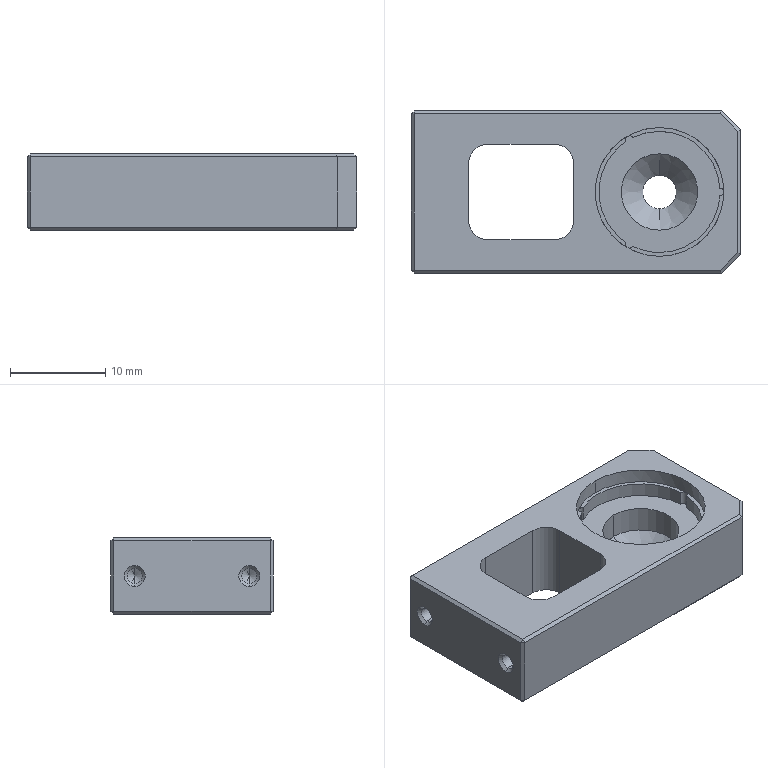NC program | NX | posted with a generic post | part box 34.5 x 17 x 8 mm
Lines 1 to 1240 of 4112:
N10 G17 G21 G94 G90
(FLOOR_WALL , TOOL : D10JING)
N12 T09 M6
N14 G54
N16 G17 G0 G90 X-27.25 Y10.497 S9500 M3
N18 G43 Z30. H9
N20 Z3.
N22 G94 G1 Z0. F1250.
N24 X-24.25
N26 X24.25
N28 Y6.248
N30 X-24.25
N32 Y1.999
N34 X24.25
N36 Y-2.251
N38 X-24.25
N40 Y-6.5
N42 X24.25
N44 X27.25
N46 Z3.
N48 G0 Z30.
N50 M5
(ZLEVEL_PROFILE , TOOL : D10)
N52 T10 M6
N54 G54
N56 G17 G0 G90 X-12.343 Y-13.6 S9500 M3
N58 G43 Z30. H10
N60 Z1.5
N62 G94 G1 X-17.504 Z1.23 F1000.
N64 X-18.913 Y-13.24 Z1.153
N66 X-20.165 Y-12.498 Z1.077
N68 X-21.248 Y-11.415 Z0.997
N70 X-21.99 Y-10.163 Z0.921
N72 X-22.35 Y-8.754 Z0.844
N74 Y8.754 Z-0.073
N76 X-21.99 Y10.163 Z-0.149
N78 X-21.248 Y11.415 Z-0.226
N80 X-20.165 Y12.498 Z-0.306
N82 X-18.913 Y13.24 Z-0.382
N84 X-17.504 Y13.6 Z-0.458
N86 X-16.95 Z-0.488
N88 X15.25 F2500.
N90 G2 X18.856 Y12.106 R5.1
N92 G1 X20.856 Y10.106
N94 G2 X22.35 Y6.5 R5.1
N96 G1 Y-6.5
N98 G2 X20.856 Y-10.106 R5.1
N100 G1 X18.856 Y-12.106
N102 G2 X15.25 Y-13.6 R5.1
N104 G1 X-16.95
N106 G2 X-20.556 Y-12.106 R5.1
N108 G1 X-20.856 Y-11.806
N110 G2 X-22.35 Y-8.2 R5.1
N112 G1 Y8.2
N114 G2 X-20.856 Y11.806 R5.1
N116 G1 X-20.556 Y12.106
N118 G2 X-16.95 Y13.6 R5.1
N120 G1 X10.979 Z-0.975
N122 X15.25
N124 G2 X18.856 Y12.106 R5.1
N126 G1 X20.856 Y10.106
N128 G2 X22.35 Y6.5 R5.1
N130 G1 Y-6.5
N132 G2 X20.856 Y-10.106 R5.1
N134 G1 X18.856 Y-12.106
N136 G2 X15.25 Y-13.6 R5.1
N138 G1 X-16.95
N140 G2 X-20.556 Y-12.106 R5.1
N142 G1 X-20.856 Y-11.806
N144 G2 X-22.35 Y-8.2 R5.1
N146 G1 Y8.2
N148 G2 X-20.856 Y11.806 R5.1
N150 G1 X-20.556 Y12.106
N152 G2 X-16.95 Y13.6 R5.1
N154 G1 X10.979 Z-1.463
N156 X15.25
N158 G2 X18.856 Y12.106 R5.1
N160 G1 X20.856 Y10.106
N162 G2 X22.35 Y6.5 R5.1
N164 G1 Y-6.5
N166 G2 X20.856 Y-10.106 R5.1
N168 G1 X18.856 Y-12.106
N170 G2 X15.25 Y-13.6 R5.1
N172 G1 X-16.95
N174 G2 X-20.556 Y-12.106 R5.1
N176 G1 X-20.856 Y-11.806
N178 G2 X-22.35 Y-8.2 R5.1
N180 G1 Y8.2
N182 G2 X-20.856 Y11.806 R5.1
N184 G1 X-20.556 Y12.106
N186 G2 X-16.95 Y13.6 R5.1
N188 G1 X10.979 Z-1.95
N190 X15.25
N192 G2 X18.856 Y12.106 R5.1
N194 G1 X20.856 Y10.106
N196 G2 X22.35 Y6.5 R5.1
N198 G1 Y-6.5
N200 G2 X20.856 Y-10.106 R5.1
N202 G1 X18.856 Y-12.106
N204 G2 X15.25 Y-13.6 R5.1
N206 G1 X-16.95
N208 G2 X-20.556 Y-12.106 R5.1
N210 G1 X-20.856 Y-11.806
N212 G2 X-22.35 Y-8.2 R5.1
N214 G1 Y8.2
N216 G2 X-20.856 Y11.806 R5.1
N218 G1 X-20.556 Y12.106
N220 G2 X-16.95 Y13.6 R5.1
N222 G1 X10.979 Z-2.438
N224 X15.25
N226 G2 X18.856 Y12.106 R5.1
N228 G1 X20.856 Y10.106
N230 G2 X22.35 Y6.5 R5.1
N232 G1 Y-6.5
N234 G2 X20.856 Y-10.106 R5.1
N236 G1 X18.856 Y-12.106
N238 G2 X15.25 Y-13.6 R5.1
N240 G1 X-16.95
N242 G2 X-20.556 Y-12.106 R5.1
N244 G1 X-20.856 Y-11.806
N246 G2 X-22.35 Y-8.2 R5.1
N248 G1 Y8.2
N250 G2 X-20.856 Y11.806 R5.1
N252 G1 X-20.556 Y12.106
N254 G2 X-16.95 Y13.6 R5.1
N256 G1 X10.979 Z-2.925
N258 X15.25
N260 G2 X18.856 Y12.106 R5.1
N262 G1 X20.856 Y10.106
N264 G2 X22.35 Y6.5 R5.1
N266 G1 Y-6.5
N268 G2 X20.856 Y-10.106 R5.1
N270 G1 X18.856 Y-12.106
N272 G2 X15.25 Y-13.6 R5.1
N274 G1 X-16.95
N276 G2 X-20.556 Y-12.106 R5.1
N278 G1 X-20.856 Y-11.806
N280 G2 X-22.35 Y-8.2 R5.1
N282 G1 Y8.2
N284 G2 X-20.856 Y11.806 R5.1
N286 G1 X-20.556 Y12.106
N288 G2 X-16.95 Y13.6 R5.1
N290 G1 X10.979 Z-3.413
N292 X15.25
N294 G2 X18.856 Y12.106 R5.1
N296 G1 X20.856 Y10.106
N298 G2 X22.35 Y6.5 R5.1
N300 G1 Y-6.5
N302 G2 X20.856 Y-10.106 R5.1
N304 G1 X18.856 Y-12.106
N306 G2 X15.25 Y-13.6 R5.1
N308 G1 X-16.95
N310 G2 X-20.556 Y-12.106 R5.1
N312 G1 X-20.856 Y-11.806
N314 G2 X-22.35 Y-8.2 R5.1
N316 G1 Y8.2
N318 G2 X-20.856 Y11.806 R5.1
N320 G1 X-20.556 Y12.106
N322 G2 X-16.95 Y13.6 R5.1
N324 G1 X10.979 Z-3.9
N326 X15.25
N328 G2 X18.856 Y12.106 R5.1
N330 G1 X20.856 Y10.106
N332 G2 X22.35 Y6.5 R5.1
N334 G1 Y-6.5
N336 G2 X20.856 Y-10.106 R5.1
N338 G1 X18.856 Y-12.106
N340 G2 X15.25 Y-13.6 R5.1
N342 G1 X-16.95
N344 G2 X-20.556 Y-12.106 R5.1
N346 G1 X-20.856 Y-11.806
N348 G2 X-22.35 Y-8.2 R5.1
N350 G1 Y8.2
N352 G2 X-20.856 Y11.806 R5.1
N354 G1 X-20.556 Y12.106
N356 G2 X-16.95 Y13.6 R5.1
N358 G1 X10.979 Z-4.388
N360 X15.25
N362 G2 X18.856 Y12.106 R5.1
N364 G1 X20.856 Y10.106
N366 G2 X22.35 Y6.5 R5.1
N368 G1 Y-6.5
N370 G2 X20.856 Y-10.106 R5.1
N372 G1 X18.856 Y-12.106
N374 G2 X15.25 Y-13.6 R5.1
N376 G1 X-16.95
N378 G2 X-20.556 Y-12.106 R5.1
N380 G1 X-20.856 Y-11.806
N382 G2 X-22.35 Y-8.2 R5.1
N384 G1 Y8.2
N386 G2 X-20.856 Y11.806 R5.1
N388 G1 X-20.556 Y12.106
N390 G2 X-16.95 Y13.6 R5.1
N392 G1 X10.979 Z-4.875
N394 X15.25
N396 G2 X18.856 Y12.106 R5.1
N398 G1 X20.856 Y10.106
N400 G2 X22.35 Y6.5 R5.1
N402 G1 Y-6.5
N404 G2 X20.856 Y-10.106 R5.1
N406 G1 X18.856 Y-12.106
N408 G2 X15.25 Y-13.6 R5.1
N410 G1 X-16.95
N412 G2 X-20.556 Y-12.106 R5.1
N414 G1 X-20.856 Y-11.806
N416 G2 X-22.35 Y-8.2 R5.1
N418 G1 Y8.2
N420 G2 X-20.856 Y11.806 R5.1
N422 G1 X-20.556 Y12.106
N424 G2 X-16.95 Y13.6 R5.1
N426 G1 X10.979 Z-5.363
N428 X15.25
N430 G2 X18.856 Y12.106 R5.1
N432 G1 X20.856 Y10.106
N434 G2 X22.35 Y6.5 R5.1
N436 G1 Y-6.5
N438 G2 X20.856 Y-10.106 R5.1
N440 G1 X18.856 Y-12.106
N442 G2 X15.25 Y-13.6 R5.1
N444 G1 X-16.95
N446 G2 X-20.556 Y-12.106 R5.1
N448 G1 X-20.856 Y-11.806
N450 G2 X-22.35 Y-8.2 R5.1
N452 G1 Y8.2
N454 G2 X-20.856 Y11.806 R5.1
N456 G1 X-20.556 Y12.106
N458 G2 X-16.95 Y13.6 R5.1
N460 G1 X10.979 Z-5.85
N462 X15.25
N464 G2 X18.856 Y12.106 R5.1
N466 G1 X20.856 Y10.106
N468 G2 X22.35 Y6.5 R5.1
N470 G1 Y-6.5
N472 G2 X20.856 Y-10.106 R5.1
N474 G1 X18.856 Y-12.106
N476 G2 X15.25 Y-13.6 R5.1
N478 G1 X-16.95
N480 G2 X-20.556 Y-12.106 R5.1
N482 G1 X-20.856 Y-11.806
N484 G2 X-22.35 Y-8.2 R5.1
N486 G1 Y8.2
N488 G2 X-20.856 Y11.806 R5.1
N490 G1 X-20.556 Y12.106
N492 G2 X-16.95 Y13.6 R5.1
N494 G1 X10.979 Z-6.338
N496 X15.25
N498 G2 X18.856 Y12.106 R5.1
N500 G1 X20.856 Y10.106
N502 G2 X22.35 Y6.5 R5.1
N504 G1 Y-6.5
N506 G2 X20.856 Y-10.106 R5.1
N508 G1 X18.856 Y-12.106
N510 G2 X15.25 Y-13.6 R5.1
N512 G1 X-16.95
N514 G2 X-20.556 Y-12.106 R5.1
N516 G1 X-20.856 Y-11.806
N518 G2 X-22.35 Y-8.2 R5.1
N520 G1 Y8.2
N522 G2 X-20.856 Y11.806 R5.1
N524 G1 X-20.556 Y12.106
N526 G2 X-16.95 Y13.6 R5.1
N528 G1 X10.979 Z-6.825
N530 X15.25
N532 G2 X18.856 Y12.106 R5.1
N534 G1 X20.856 Y10.106
N536 G2 X22.35 Y6.5 R5.1
N538 G1 Y-6.5
N540 G2 X20.856 Y-10.106 R5.1
N542 G1 X18.856 Y-12.106
N544 G2 X15.25 Y-13.6 R5.1
N546 G1 X-16.95
N548 G2 X-20.556 Y-12.106 R5.1
N550 G1 X-20.856 Y-11.806
N552 G2 X-22.35 Y-8.2 R5.1
N554 G1 Y8.2
N556 G2 X-20.856 Y11.806 R5.1
N558 G1 X-20.556 Y12.106
N560 G2 X-16.95 Y13.6 R5.1
N562 G1 X10.979 Z-7.313
N564 X15.25
N566 G2 X18.856 Y12.106 R5.1
N568 G1 X20.856 Y10.106
N570 G2 X22.35 Y6.5 R5.1
N572 G1 Y-6.5
N574 G2 X20.856 Y-10.106 R5.1
N576 G1 X18.856 Y-12.106
N578 G2 X15.25 Y-13.6 R5.1
N580 G1 X-16.95
N582 G2 X-20.556 Y-12.106 R5.1
N584 G1 X-20.856 Y-11.806
N586 G2 X-22.35 Y-8.2 R5.1
N588 G1 Y8.2
N590 G2 X-20.856 Y11.806 R5.1
N592 G1 X-20.556 Y12.106
N594 G2 X-16.95 Y13.6 R5.1
N596 G1 X10.979 Z-7.8
N598 X15.25
N600 G2 X18.856 Y12.106 R5.1
N602 G1 X20.856 Y10.106
N604 G2 X22.35 Y6.5 R5.1
N606 G1 Y-6.5
N608 G2 X20.856 Y-10.106 R5.1
N610 G1 X18.856 Y-12.106
N612 G2 X15.25 Y-13.6 R5.1
N614 G1 X-16.95
N616 G2 X-20.556 Y-12.106 R5.1
N618 G1 X-20.856 Y-11.806
N620 G2 X-22.35 Y-8.2 R5.1
N622 G1 Y8.2
N624 G2 X-20.856 Y11.806 R5.1
N626 G1 X-20.556 Y12.106
N628 G2 X-16.95 Y13.6 R5.1
N630 G1 X10.979
N632 Z-6.3
N634 G0 Z30.
(HOLE_MILLING , TOOL : D10)
N636 X8.75 Y0.
N638 Z0.5
N640 G3 X9.575 Y-0.825 R0.825 F2000.
N642 X10.4 Y0. R0.825
N644 X10.4 Y0. Z0. I-1.65 J0.
N646 X10.4 Y0. Z-0.5 I-1.65 J0.
N648 X10.4 Y0. Z-1. I-1.65 J0.
N650 X10.4 Y0. Z-1.5 I-1.65 J0.
N652 X8.75 Y1.65 R1.65
N654 X10.4 Y0. R-1.65
N656 X9.575 Y0.825 R0.825
N658 X8.75 Y0. R0.825
N660 G0 Z30.
(HOLE_MILLING_COPY , TOOL : D10)
N662 Z-1.
N664 G3 X9.375 Y-0.625 R0.625
N666 X10. Y0. R0.625
N668 X10. Y0. Z-1.5 I-1.25 J0.
N670 X10. Y0. Z-2. I-1.25 J0.
N672 X10. Y0. Z-2.5 I-1.25 J0.
N674 X10. Y0. Z-3. I-1.25 J0.
N676 X8.75 Y1.25 R1.25
N678 X10. Y0. R-1.25
N680 X9.375 Y0.625 R0.625
N682 X8.75 Y0. R0.625
N684 G0 Z30.
N686 M5
(ZLEVEL_PROFILE_COPY_COPY , TOOL : D4)
N688 T04 M6
N690 G54
N692 G17 G0 G90 X-3.25 Y1.754 S9500 M3
N694 G43 Z30. H4
N696 Z1.5
N698 G94 G1 Y2.002 Z1.487 F1000.
N700 X-3.298 Y2. Z1.485
N702 X-8.202 Z1.227
N704 X-8.25 Y2.002 Z1.225
N706 Y-2. Z1.015
N708 X-3.25 Z0.753
N710 Y2.002 Z0.544
N712 X-3.298 Y2. Z0.541
N714 X-8.202 Z0.284
N716 X-8.25 Y2.002 Z0.281
N718 Y-2. Z0.072
N720 X-3.25 Z-0.19
N722 Y2.002 Z-0.4
N724 X-3.298 Y2. F2000.
N726 X-8.202
N728 X-8.25 Y2.002
N730 Y-2.
N732 X-3.25
N734 Y2.002
N736 X-3.423 Y2. Z-0.405
N738 X-8.097 Z-0.544
N740 X-8.25 Y1.982 Z-0.549
N742 Y-2. Z-0.667
N744 X-8.077 Z-0.672
N746 X-3.749 Z-0.8
N748 X-3.25
N750 Y2.002
N752 X-3.423 Y2. Z-0.805
N754 X-8.097 Z-0.944
N756 X-8.25 Y1.982 Z-0.949
N758 Y-2. Z-1.067
N760 X-8.077 Z-1.072
N762 X-3.749 Z-1.2
N764 X-3.25
N766 Y2.002
N768 X-3.423 Y2. Z-1.205
N770 X-8.097 Z-1.344
N772 X-8.25 Y1.982 Z-1.349
N774 Y-2. Z-1.467
N776 X-8.077 Z-1.472
N778 X-3.749 Z-1.6
N780 X-3.25
N782 Y2.002
N784 X-3.423 Y2. Z-1.605
N786 X-8.097 Z-1.744
N788 X-8.25 Y1.982 Z-1.749
N790 Y-2. Z-1.867
N792 X-8.077 Z-1.872
N794 X-3.749 Z-2.
N796 X-3.25
N798 Y2.002
N800 X-3.423 Y2. Z-2.005
N802 X-8.097 Z-2.144
N804 X-8.25 Y1.982 Z-2.149
N806 Y-2. Z-2.267
N808 X-8.077 Z-2.272
N810 X-3.749 Z-2.4
N812 X-3.25
N814 Y2.002
N816 X-3.423 Y2. Z-2.405
N818 X-8.097 Z-2.544
N820 X-8.25 Y1.982 Z-2.549
N822 Y-2. Z-2.667
N824 X-8.077 Z-2.672
N826 X-3.749 Z-2.8
N828 X-3.25
N830 Y2.002
N832 X-3.423 Y2. Z-2.805
N834 X-8.097 Z-2.944
N836 X-8.25 Y1.982 Z-2.949
N838 Y-2. Z-3.067
N840 X-8.077 Z-3.072
N842 X-3.749 Z-3.2
N844 X-3.25
N846 Y2.002
N848 X-3.423 Y2. Z-3.205
N850 X-8.097 Z-3.344
N852 X-8.25 Y1.982 Z-3.349
N854 Y-2. Z-3.467
N856 X-8.077 Z-3.472
N858 X-3.749 Z-3.6
N860 X-3.25
N862 Y2.002
N864 X-3.423 Y2. Z-3.605
N866 X-8.097 Z-3.744
N868 X-8.25 Y1.982 Z-3.749
N870 Y-2. Z-3.867
N872 X-8.077 Z-3.872
N874 X-3.749 Z-4.
N876 X-3.25
N878 Y2.002
N880 X-3.423 Y2. Z-4.005
N882 X-8.097 Z-4.144
N884 X-8.25 Y1.982 Z-4.149
N886 Y-2. Z-4.267
N888 X-8.077 Z-4.272
N890 X-3.749 Z-4.4
N892 X-3.25
N894 Y2.002
N896 X-3.423 Y2. Z-4.405
N898 X-8.097 Z-4.544
N900 X-8.25 Y1.982 Z-4.549
N902 Y-2. Z-4.667
N904 X-8.077 Z-4.672
N906 X-3.749 Z-4.8
N908 X-3.25
N910 Y2.002
N912 X-3.423 Y2. Z-4.805
N914 X-8.097 Z-4.944
N916 X-8.25 Y1.982 Z-4.949
N918 Y-2. Z-5.067
N920 X-8.077 Z-5.072
N922 X-3.749 Z-5.2
N924 X-3.25
N926 Y2.002
N928 X-3.423 Y2. Z-5.205
N930 X-8.097 Z-5.344
N932 X-8.25 Y1.982 Z-5.349
N934 Y-2. Z-5.467
N936 X-8.077 Z-5.472
N938 X-3.749 Z-5.6
N940 X-3.25
N942 Y2.002
N944 X-3.423 Y2. Z-5.605
N946 X-8.097 Z-5.744
N948 X-8.25 Y1.982 Z-5.749
N950 Y-2. Z-5.867
N952 X-8.077 Z-5.872
N954 X-3.749 Z-6.
N956 X-3.25
N958 Y2.002
N960 X-3.423 Y2. Z-6.005
N962 X-8.097 Z-6.144
N964 X-8.25 Y1.982 Z-6.149
N966 Y-2. Z-6.267
N968 X-8.077 Z-6.272
N970 X-3.749 Z-6.4
N972 X-3.25
N974 Y2.002
N976 X-3.423 Y2. Z-6.405
N978 X-8.097 Z-6.544
N980 X-8.25 Y1.982 Z-6.549
N982 Y-2. Z-6.667
N984 X-8.077 Z-6.672
N986 X-3.749 Z-6.8
N988 X-3.25
N990 Y2.002
N992 X-3.423 Y2. Z-6.805
N994 X-8.097 Z-6.944
N996 X-8.25 Y1.981 Z-6.949
N998 Y-2. Z-7.067
N1000 X-8.077 Z-7.072
N1002 X-3.749 Z-7.2
N1004 X-3.25
N1006 Y2.002
N1008 X-3.423 Y2. Z-7.205
N1010 X-8.097 Z-7.344
N1012 X-8.25 Y1.981 Z-7.349
N1014 Y-2. Z-7.467
N1016 X-8.077 Z-7.472
N1018 X-3.749 Z-7.6
N1020 X-3.25
N1022 Y2.002
N1024 X-3.423 Y2. Z-7.605
N1026 X-8.097 Z-7.744
N1028 X-8.25 Y1.981 Z-7.749
N1030 Y-2. Z-7.867
N1032 X-8.077 Z-7.872
N1034 X-3.749 Z-8.
N1036 X-3.25
N1038 Y2.002
N1040 X-3.298 Y2.
N1042 X-8.202
N1044 X-8.25 Y2.002
N1046 Y-2.
N1048 X-3.749
N1050 Z-6.5
N1052 G0 Z30.
(ZLEVEL_PROFILE_COPY_COPY_COPY , TOOL : D4)
N1054 X-7.596 Y-2.9
N1056 Z1.5
N1058 G1 X-2.35 Z1.225 F1000.
N1060 Y2.903 Z0.921
N1062 X-2.39 Y2.9 Z0.919
N1064 X-9.11 Z0.567
N1066 X-9.15 Y2.903 Z0.565
N1068 Y-2.9 Z0.26
N1070 X-2.35 Z-0.096
N1072 Y2.903 Z-0.4
N1074 X-2.39 Y2.9 F2000.
N1076 X-9.11
N1078 X-9.15 Y2.903
N1080 Y-2.9
N1082 X-2.35
N1084 Y2.903
N1086 X-2.494 Y2.9 Z-0.403
N1088 X-8.988 Z-0.54
N1090 X-9.132 Y2.901 Z-0.544
N1092 X-9.15 Y2.776 Z-0.547
N1094 Y-2.852 Z-0.666
N1096 X-9.054 Y-2.9 Z-0.669
N1098 X-2.849 Z-0.8
N1100 X-2.35
N1102 Y2.903
N1104 X-2.494 Y2.9 Z-0.803
N1106 X-8.988 Z-0.94
N1108 X-9.132 Y2.901 Z-0.944
N1110 X-9.15 Y2.776 Z-0.947
N1112 Y-2.852 Z-1.066
N1114 X-9.054 Y-2.9 Z-1.069
N1116 X-2.849 Z-1.2
N1118 X-2.35
N1120 Y2.903
N1122 X-2.494 Y2.9 Z-1.203
N1124 X-8.988 Z-1.34
N1126 X-9.132 Y2.901 Z-1.344
N1128 X-9.15 Y2.776 Z-1.347
N1130 Y-2.852 Z-1.466
N1132 X-9.054 Y-2.9 Z-1.469
N1134 X-2.849 Z-1.6
N1136 X-2.35
N1138 Y2.902
N1140 X-2.494 Y2.9 Z-1.603
N1142 X-8.988 Z-1.74
N1144 X-9.132 Y2.901 Z-1.744
N1146 X-9.15 Y2.776 Z-1.747
N1148 Y-2.852 Z-1.866
N1150 X-9.054 Y-2.9 Z-1.869
N1152 X-2.849 Z-2.
N1154 X-2.35
N1156 Y2.902
N1158 X-2.494 Y2.9 Z-2.003
N1160 X-8.988 Z-2.14
N1162 X-9.132 Y2.901 Z-2.144
N1164 X-9.15 Y2.776 Z-2.147
N1166 Y-2.852 Z-2.266
N1168 X-9.054 Y-2.9 Z-2.269
N1170 X-2.849 Z-2.4
N1172 X-2.35
N1174 Y2.902
N1176 X-2.494 Y2.9 Z-2.403
N1178 X-8.988 Z-2.54
N1180 X-9.132 Y2.901 Z-2.544
N1182 X-9.15 Y2.776 Z-2.547
N1184 Y-2.852 Z-2.666
N1186 X-9.054 Y-2.9 Z-2.669
N1188 X-2.849 Z-2.8
N1190 X-2.35
N1192 Y2.902
N1194 X-2.494 Y2.9 Z-2.803
N1196 X-8.988 Z-2.94
N1198 X-9.132 Y2.901 Z-2.944
N1200 X-9.15 Y2.776 Z-2.947
N1202 Y-2.852 Z-3.066
N1204 X-9.054 Y-2.9 Z-3.069
N1206 X-2.849 Z-3.2
N1208 X-2.35
N1210 Y2.902
N1212 X-2.494 Y2.9 Z-3.203
N1214 X-8.988 Z-3.34
N1216 X-9.132 Y2.901 Z-3.344
N1218 X-9.15 Y2.776 Z-3.347
N1220 Y-2.852 Z-3.466
N1222 X-9.054 Y-2.9 Z-3.469
N1224 X-2.849 Z-3.6
N1226 X-2.35
N1228 Y2.902
N1230 X-2.494 Y2.9 Z-3.603
N1232 X-8.988 Z-3.74
N1234 X-9.132 Y2.901 Z-3.744
N1236 X-9.15 Y2.776 Z-3.747
N1238 Y-2.852 Z-3.866
N1240 X-9.054 Y-2.9 Z-3.869
N1242 X-2.849 Z-4.
N1244 X-2.35
N1246 Y2.902
N1248 X-2.494 Y2.9 Z-4.003
N1250 X-8.988 Z-4.14
N1252 X-9.132 Y2.901 Z-4.144
N1254 X-9.15 Y2.776 Z-4.147
N1256 Y-2.852 Z-4.266
N1258 X-9.054 Y-2.9 Z-4.269
N1260 X-2.849 Z-4.4
N1262 X-2.35
N1264 Y2.902
N1266 X-2.494 Y2.9 Z-4.403
N1268 X-8.988 Z-4.54
N1270 X-9.132 Y2.901 Z-4.544
N1272 X-9.15 Y2.776 Z-4.547
N1274 Y-2.852 Z-4.666
N1276 X-9.054 Y-2.9 Z-4.669
N1278 X-2.849 Z-4.8
N1280 X-2.35
N1282 Y2.902
N1284 X-2.494 Y2.9 Z-4.803
N1286 X-8.988 Z-4.94
N1288 X-9.132 Y2.901 Z-4.944
N1290 X-9.15 Y2.776 Z-4.947
N1292 Y-2.852 Z-5.066
N1294 X-9.054 Y-2.9 Z-5.069
N1296 X-2.849 Z-5.2
N1298 X-2.35
N1300 Y2.902
N1302 X-2.494 Y2.9 Z-5.203
N1304 X-8.988 Z-5.34
N1306 X-9.132 Y2.901 Z-5.344
N1308 X-9.15 Y2.776 Z-5.347
N1310 Y-2.852 Z-5.466
N1312 X-9.054 Y-2.9 Z-5.469
N1314 X-2.849 Z-5.6
N1316 X-2.35
N1318 Y2.902
N1320 X-2.494 Y2.9 Z-5.603
N1322 X-8.988 Z-5.74
N1324 X-9.132 Y2.901 Z-5.744
N1326 X-9.15 Y2.776 Z-5.747
N1328 Y-2.852 Z-5.866
N1330 X-9.054 Y-2.9 Z-5.869
N1332 X-2.849 Z-6.
N1334 X-2.35
N1336 Y2.902
N1338 X-2.494 Y2.9 Z-6.003
N1340 X-8.988 Z-6.14
N1342 X-9.132 Y2.901 Z-6.144
N1344 X-9.15 Y2.776 Z-6.147
N1346 Y-2.852 Z-6.266
N1348 X-9.054 Y-2.9 Z-6.269
N1350 X-2.849 Z-6.4
N1352 X-2.35
N1354 Y2.902
N1356 X-2.494 Y2.9 Z-6.403
N1358 X-8.988 Z-6.54
N1360 X-9.132 Y2.901 Z-6.544
N1362 X-9.15 Y2.776 Z-6.547
N1364 Y-2.852 Z-6.666
N1366 X-9.054 Y-2.9 Z-6.669
N1368 X-2.849 Z-6.8
N1370 X-2.35
N1372 Y2.902
N1374 X-2.494 Y2.9 Z-6.803
N1376 X-8.988 Z-6.94
N1378 X-9.132 Y2.901 Z-6.944
N1380 X-9.15 Y2.776 Z-6.947
N1382 Y-2.852 Z-7.066
N1384 X-9.054 Y-2.9 Z-7.069
N1386 X-2.849 Z-7.2
N1388 X-2.35
N1390 Y2.902
N1392 X-2.494 Y2.9 Z-7.203
N1394 X-8.988 Z-7.34
N1396 X-9.132 Y2.901 Z-7.344
N1398 X-9.15 Y2.776 Z-7.347
N1400 Y-2.852 Z-7.466
N1402 X-9.054 Y-2.9 Z-7.469
N1404 X-2.849 Z-7.6
N1406 X-2.35
N1408 Y2.902
N1410 X-2.494 Y2.9 Z-7.603
N1412 X-8.988 Z-7.74
N1414 X-9.132 Y2.901 Z-7.744
N1416 X-9.15 Y2.776 Z-7.747
N1418 Y-2.852 Z-7.866
N1420 X-9.054 Y-2.9 Z-7.869
N1422 X-2.849 Z-8.
N1424 X-2.35
N1426 Y2.902
N1428 X-2.39 Y2.9
N1430 X-9.11
N1432 X-9.15 Y2.902
N1434 Y-2.9
N1436 X-2.849
N1438 Z-6.5
N1440 G0 Z30.
(ZLEVEL_PROFILE_COPY_COPY_COPY_COPY_1 , TOOL : D4)
N1442 X9.088 Y1.869
N1444 Z-1.5
N1446 G1 X8.949 Y1.9 Z-1.507 F1000.
N1448 X8.75 Z-1.518
N1450 X8.555 Z-1.528
N1452 X8.12 Y1.803 Z-1.551
N1454 X7.719 Y1.608 Z-1.575
N1456 X7.375 Y1.326 Z-1.598
N1458 X7.105 Y0.971 Z-1.622
N1460 X6.942 Y0.616 Z-1.642
N1462 X6.845 Y0.136 Z-1.668
N1464 X6.873 Y-0.352 Z-1.693
N1466 X7.024 Y-0.818 Z-1.719
N1468 X7.289 Y-1.23 Z-1.745
N1470 X7.649 Y-1.561 Z-1.77
N1472 X8.082 Y-1.789 Z-1.796
N1474 X8.559 Y-1.9 Z-1.822
N1476 X8.949 Z-1.842
N1478 X9.434 Y-1.783 Z-1.868
N1480 X9.873 Y-1.545 Z-1.894
N1482 X10.235 Y-1.201 Z-1.92
N1484 X10.495 Y-0.776 Z-1.947
N1486 X10.637 Y-0.297 Z-1.973
N1488 X10.649 Y0.202 Z-1.999
N1490 X10.532 Y0.687 Z-2.025
N1492 X10.355 Y1.035 Z-2.046
N1494 X10.086 Y1.365 Z-2.068
N1496 X9.75 Y1.627 Z-2.09
N1498 X9.365 Y1.808 Z-2.112
N1500 X8.949 Y1.9 Z-2.135
N1502 X8.75 Z-2.145
N1504 X8.555 Z-2.155
N1506 X8.12 Y1.803 Z-2.179
N1508 X7.719 Y1.608 Z-2.202
N1510 X7.375 Y1.326 Z-2.226
N1512 X7.105 Y0.971 Z-2.249
N1514 X6.942 Y0.616 Z-2.269
N1516 X6.845 Y0.136 Z-2.295
N1518 X6.873 Y-0.352 Z-2.321
N1520 X7.024 Y-0.818 Z-2.346
N1522 X7.289 Y-1.23 Z-2.372
N1524 X7.649 Y-1.561 Z-2.398
N1526 X8.082 Y-1.789 Z-2.423
N1528 X8.559 Y-1.9 Z-2.449
N1530 X8.949 Z-2.469
N1532 X9.434 Y-1.783 Z-2.496
N1534 X9.873 Y-1.545 Z-2.522
N1536 X10.235 Y-1.201 Z-2.548
N1538 X10.495 Y-0.776 Z-2.574
N1540 X10.637 Y-0.297 Z-2.6
N1542 X10.649 Y0.202 Z-2.626
N1544 X10.532 Y0.687 Z-2.652
N1546 X10.355 Y1.035 Z-2.673
N1548 X10.086 Y1.365 Z-2.695
N1550 X9.75 Y1.627 Z-2.718
N1552 X9.365 Y1.808 Z-2.74
N1554 X8.949 Y1.9 Z-2.762
N1556 X8.75 Z-2.773
N1558 X8.555 Z-2.783
N1560 X8.12 Y1.803 Z-2.806
N1562 X7.719 Y1.608 Z-2.83
N1564 X7.375 Y1.326 Z-2.853
N1566 X7.105 Y0.971 Z-2.876
N1568 X6.942 Y0.616 Z-2.897
N1570 X6.845 Y0.136 Z-2.922
N1572 X6.873 Y-0.352 Z-2.948
N1574 X7.024 Y-0.818 Z-2.974
N1576 X7.289 Y-1.23 Z-2.999
N1578 X7.649 Y-1.561 Z-3.025
N1580 X8.082 Y-1.789 Z-3.051
N1582 X8.559 Y-1.9 Z-3.076
N1584 X8.949 Z-3.097
N1586 X9.434 Y-1.783 Z-3.123
N1588 X9.873 Y-1.545 Z-3.149
N1590 X10.235 Y-1.201 Z-3.175
N1592 X10.495 Y-0.776 Z-3.201
N1594 X10.637 Y-0.297 Z-3.228
N1596 X10.649 Y0.202 Z-3.254
N1598 X10.532 Y0.687 Z-3.28
N1600 X10.355 Y1.035 Z-3.3
N1602 X10.086 Y1.365 Z-3.323
N1604 X9.75 Y1.627 Z-3.345
N1606 X9.365 Y1.808 Z-3.367
N1608 X8.949 Y1.9 Z-3.39
N1610 X8.75 Z-3.4
N1612 G3 X6.85 Y0. R1.9 F2000.
N1614 X8.75 Y1.9 R-1.9
N1616 G1 X8.607 Y1.885 Z-3.406
N1618 X8.463 Y1.872 Z-3.413
N1620 X8.322 Y1.843 Z-3.419
N1622 X8.184 Y1.805 Z-3.426
N1624 X8.048 Y1.757 Z-3.432
N1626 X7.917 Y1.698 Z-3.439
N1628 X7.789 Y1.632 Z-3.445
N1630 X7.67 Y1.552 Z-3.452
N1632 X7.552 Y1.469 Z-3.458
N1634 X7.447 Y1.37 Z-3.465
N1636 X7.345 Y1.269 Z-3.471
N1638 X7.254 Y1.158 Z-3.477
N1640 X7.17 Y1.041 Z-3.484
N1642 X7.095 Y0.918 Z-3.49
N1644 X7.032 Y0.79 Z-3.497
N1646 X6.974 Y0.658 Z-3.503
N1648 X6.932 Y0.52 Z-3.51
N1650 X6.894 Y0.381 Z-3.516
N1652 X6.874 Y0.239 Z-3.523
N1654 X6.859 Y0.096 Z-3.529
N1656 Y-0.048 Z-3.535
N1658 X6.868 Y-0.191 Z-3.542
N1660 X6.887 Y-0.334 Z-3.548
N1662 X6.919 Y-0.474 Z-3.555
N1664 X6.958 Y-0.612 Z-3.561
N1666 X7.012 Y-0.746 Z-3.568
N1668 X7.07 Y-0.877 Z-3.574
N1670 X7.145 Y-1. Z-3.581
N1672 X7.224 Y-1.12 Z-3.587
N1674 X7.315 Y-1.232 Z-3.594
N1676 X7.412 Y-1.338 Z-3.6
N1678 X7.517 Y-1.436 Z-3.606
N1680 X7.631 Y-1.525 Z-3.613
N1682 X7.748 Y-1.608 Z-3.619
N1684 X7.875 Y-1.676 Z-3.626
N1686 X8.003 Y-1.741 Z-3.632
N1688 X8.138 Y-1.789 Z-3.639
N1690 X8.275 Y-1.833 Z-3.645
N1692 X8.416 Y-1.862 Z-3.652
N1694 X8.559 Y-1.882 Z-3.658
N1696 X8.702 Y-1.892 Z-3.665
N1698 X8.846 Y-1.889 Z-3.671
N1700 X8.989 Y-1.879 Z-3.677
N1702 X9.131 Y-1.852 Z-3.684
N1704 X9.271 Y-1.821 Z-3.69
N1706 X9.407 Y-1.773 Z-3.697
N1708 X9.54 Y-1.72 Z-3.703
N1710 X9.668 Y-1.654 Z-3.71
N1712 X9.791 Y-1.58 Z-3.716
N1714 X9.908 Y-1.497 Z-3.723
N1716 X10.018 Y-1.403 Z-3.729
N1718 X10.123 Y-1.305 Z-3.735
N1720 X10.216 Y-1.195 Z-3.742
N1722 X10.305 Y-1.082 Z-3.748
N1724 X10.38 Y-0.959 Z-3.755
N1726 X10.45 Y-0.834 Z-3.761
N1728 X10.507 Y-0.702 Z-3.768
N1730 X10.555 Y-0.566 Z-3.774
N1732 X10.593 Y-0.428 Z-3.781
N1734 X10.619 Y-0.286 Z-3.787
N1736 X10.639 Y-0.143 Z-3.794
N1738 X10.65 Y0. Z-3.8
N1740 G3 X8.75 Y1.9 R1.9
N1742 G1 X8.607 Y1.886 Z-3.806
N1744 X8.463 Y1.872 Z-3.813
N1746 X8.323 Y1.842 Z-3.819
N1748 X8.184 Y1.805 Z-3.826
N1750 X8.048 Y1.757 Z-3.832
N1752 X7.917 Y1.698 Z-3.839
N1754 X7.79 Y1.632 Z-3.845
N1756 X7.67 Y1.552 Z-3.852
N1758 X7.552 Y1.469 Z-3.858
N1760 X7.447 Y1.37 Z-3.865
N1762 X7.345 Y1.269 Z-3.871
N1764 X7.254 Y1.158 Z-3.877
N1766 X7.17 Y1.041 Z-3.884
N1768 X7.095 Y0.918 Z-3.89
N1770 X7.032 Y0.789 Z-3.897
N1772 X6.974 Y0.658 Z-3.903
N1774 X6.932 Y0.52 Z-3.91
N1776 X6.894 Y0.381 Z-3.916
N1778 X6.875 Y0.239 Z-3.923
N1780 X6.859 Y0.096 Z-3.929
N1782 X6.86 Y-0.048 Z-3.935
N1784 X6.868 Y-0.191 Z-3.942
N1786 X6.888 Y-0.334 Z-3.948
N1788 X6.919 Y-0.474 Z-3.955
N1790 X6.958 Y-0.613 Z-3.961
N1792 X7.012 Y-0.746 Z-3.968
N1794 X7.07 Y-0.877 Z-3.974
N1796 X7.145 Y-1. Z-3.981
N1798 X7.224 Y-1.121 Z-3.987
N1800 X7.315 Y-1.232 Z-3.994
N1802 X7.412 Y-1.338 Z-4.
N1804 X7.517 Y-1.436 Z-4.006
N1806 X7.631 Y-1.524 Z-4.013
N1808 X7.748 Y-1.607 Z-4.019
N1810 X7.875 Y-1.676 Z-4.026
N1812 X8.003 Y-1.741 Z-4.032
N1814 X8.138 Y-1.789 Z-4.039
N1816 X8.276 Y-1.833 Z-4.045
N1818 X8.416 Y-1.862 Z-4.052
N1820 X8.559 Y-1.882 Z-4.058
N1822 X8.702 Y-1.892 Z-4.065
N1824 X8.846 Y-1.889 Z-4.071
N1826 X8.989 Y-1.879 Z-4.077
N1828 X9.131 Y-1.852 Z-4.084
N1830 X9.271 Y-1.821 Z-4.09
N1832 X9.407 Y-1.773 Z-4.097
N1834 X9.54 Y-1.72 Z-4.103
N1836 X9.668 Y-1.654 Z-4.11
N1838 X9.791 Y-1.579 Z-4.116
N1840 X9.908 Y-1.496 Z-4.123
N1842 X10.018 Y-1.403 Z-4.129
N1844 X10.123 Y-1.305 Z-4.135
N1846 X10.215 Y-1.195 Z-4.142
N1848 X10.305 Y-1.082 Z-4.148
N1850 X10.379 Y-0.959 Z-4.155
N1852 X10.45 Y-0.834 Z-4.161
N1854 X10.507 Y-0.702 Z-4.168
N1856 X10.555 Y-0.566 Z-4.174
N1858 X10.593 Y-0.428 Z-4.181
N1860 X10.619 Y-0.286 Z-4.187
N1862 X10.638 Y-0.143 Z-4.194
N1864 X10.65 Y0. Z-4.2
N1866 G3 X8.75 Y1.9 R1.9
N1868 G1 X8.607 Y1.886 Z-4.206
N1870 X8.463 Y1.872 Z-4.213
N1872 X8.323 Y1.842 Z-4.219
N1874 X8.184 Y1.805 Z-4.225
N1876 X8.048 Y1.757 Z-4.231
N1878 X7.917 Y1.698 Z-4.238
N1880 X7.79 Y1.632 Z-4.244
N1882 X7.67 Y1.552 Z-4.25
N1884 X7.553 Y1.469 Z-4.256
N1886 X7.447 Y1.37 Z-4.263
N1888 X7.345 Y1.269 Z-4.269
N1890 X7.254 Y1.158 Z-4.275
N1892 X7.171 Y1.041 Z-4.281
N1894 X7.095 Y0.918 Z-4.288
N1896 X7.032 Y0.789 Z-4.294
N1898 X6.974 Y0.658 Z-4.3
N1900 X6.932 Y0.52 Z-4.306
N1902 X6.894 Y0.381 Z-4.313
N1904 X6.875 Y0.239 Z-4.319
N1906 X6.859 Y0.096 Z-4.325
N1908 Y-0.048 Z-4.331
N1910 X6.868 Y-0.191 Z-4.338
N1912 X6.888 Y-0.334 Z-4.344
N1914 X6.919 Y-0.474 Z-4.35
N1916 X6.958 Y-0.613 Z-4.356
N1918 X7.013 Y-0.746 Z-4.363
N1920 X7.071 Y-0.877 Z-4.369
N1922 X7.146 Y-1. Z-4.375
N1924 X7.224 Y-1.121 Z-4.381
N1926 X7.315 Y-1.232 Z-4.388
N1928 X7.412 Y-1.338 Z-4.394
N1930 X7.517 Y-1.436 Z-4.4
N1932 X7.631 Y-1.524 Z-4.406
N1934 X7.748 Y-1.607 Z-4.413
N1936 X7.875 Y-1.676 Z-4.419
N1938 X8.003 Y-1.741 Z-4.425
N1940 X8.138 Y-1.789 Z-4.431
N1942 X8.276 Y-1.832 Z-4.438
N1944 X8.416 Y-1.862 Z-4.444
N1946 X8.559 Y-1.882 Z-4.45
N1948 X8.702 Y-1.892 Z-4.456
N1950 X8.846 Y-1.889 Z-4.463
N1952 X8.989 Y-1.879 Z-4.469
N1954 X9.131 Y-1.852 Z-4.475
N1956 X9.271 Y-1.821 Z-4.481
N1958 X9.407 Y-1.773 Z-4.488
N1960 X9.54 Y-1.72 Z-4.494
N1962 X9.668 Y-1.654 Z-4.5
N1964 X9.791 Y-1.579 Z-4.506
N1966 X9.908 Y-1.496 Z-4.513
N1968 X10.018 Y-1.403 Z-4.519
N1970 X10.123 Y-1.305 Z-4.525
N1972 X10.215 Y-1.195 Z-4.531
N1974 X10.305 Y-1.082 Z-4.538
N1976 X10.379 Y-0.959 Z-4.544
N1978 X10.449 Y-0.834 Z-4.55
N1980 X10.506 Y-0.702 Z-4.556
N1982 X10.555 Y-0.566 Z-4.563
N1984 X10.594 Y-0.428 Z-4.569
N1986 X10.619 Y-0.286 Z-4.575
N1988 X10.638 Y-0.143 Z-4.581
N1990 X10.65 Y0. Z-4.588
N1992 G3 X8.75 Y1.9 R1.9
N1994 G1 X8.607 Y1.885 Z-4.594
N1996 X8.463 Y1.872 Z-4.6
N1998 X8.323 Y1.842 Z-4.606
N2000 X8.184 Y1.805 Z-4.613
N2002 X8.048 Y1.757 Z-4.619
N2004 X7.917 Y1.698 Z-4.625
N2006 X7.79 Y1.631 Z-4.631
N2008 X7.67 Y1.552 Z-4.638
N2010 X7.553 Y1.468 Z-4.644
N2012 X7.447 Y1.37 Z-4.65
N2014 X7.345 Y1.269 Z-4.656
N2016 X7.255 Y1.158 Z-4.663
N2018 X7.17 Y1.041 Z-4.669
N2020 X7.095 Y0.918 Z-4.675
N2022 X7.032 Y0.789 Z-4.681
N2024 X6.974 Y0.658 Z-4.688
N2026 X6.932 Y0.52 Z-4.694
N2028 X6.894 Y0.381 Z-4.7
N2030 X6.874 Y0.239 Z-4.706
N2032 X6.86 Y0.096 Z-4.713
N2034 X6.859 Y-0.048 Z-4.719
N2036 X6.868 Y-0.191 Z-4.725
N2038 X6.887 Y-0.334 Z-4.731
N2040 X6.919 Y-0.474 Z-4.738
N2042 X6.958 Y-0.612 Z-4.744
N2044 X7.013 Y-0.746 Z-4.75
N2046 X7.071 Y-0.877 Z-4.756
N2048 X7.146 Y-1. Z-4.763
N2050 X7.224 Y-1.12 Z-4.769
N2052 X7.315 Y-1.232 Z-4.775
N2054 X7.413 Y-1.337 Z-4.781
N2056 X7.517 Y-1.436 Z-4.788
N2058 X7.631 Y-1.524 Z-4.794
N2060 X7.748 Y-1.607 Z-4.8
N2062 X7.875 Y-1.676 Z-4.806
N2064 X8.003 Y-1.741 Z-4.813
N2066 X8.138 Y-1.789 Z-4.819
N2068 X8.276 Y-1.832 Z-4.825
N2070 X8.416 Y-1.862 Z-4.831
N2072 X8.559 Y-1.882 Z-4.838
N2074 X8.702 Y-1.892 Z-4.844
N2076 X8.846 Y-1.889 Z-4.85
N2078 X8.989 Y-1.878 Z-4.856
N2080 X9.131 Y-1.852 Z-4.863
N2082 X9.271 Y-1.821 Z-4.869
N2084 X9.407 Y-1.773 Z-4.875
N2086 X9.54 Y-1.72 Z-4.881
N2088 X9.668 Y-1.653 Z-4.888
N2090 X9.791 Y-1.579 Z-4.894
N2092 X9.908 Y-1.496 Z-4.9
N2094 X10.018 Y-1.403 Z-4.906
N2096 X10.123 Y-1.305 Z-4.913
N2098 X10.215 Y-1.195 Z-4.919
N2100 X10.304 Y-1.082 Z-4.925
N2102 X10.379 Y-0.959 Z-4.931
N2104 X10.449 Y-0.834 Z-4.938
N2106 X10.506 Y-0.702 Z-4.944
N2108 X10.555 Y-0.566 Z-4.95
N2110 X10.594 Y-0.428 Z-4.956
N2112 X10.619 Y-0.286 Z-4.963
N2114 X10.639 Y-0.143 Z-4.969
N2116 X10.65 Y0. Z-4.975
N2118 G3 X8.75 Y1.9 R1.9
N2120 G1 X8.607 Y1.885 Z-4.981
N2122 X8.463 Y1.872 Z-4.988
N2124 X8.323 Y1.842 Z-4.994
N2126 X8.184 Y1.805 Z-5.
N2128 X8.048 Y1.757 Z-5.006
N2130 X7.917 Y1.698 Z-5.013
N2132 X7.789 Y1.632 Z-5.019
N2134 X7.67 Y1.552 Z-5.025
N2136 X7.553 Y1.468 Z-5.031
N2138 X7.447 Y1.37 Z-5.038
N2140 X7.345 Y1.269 Z-5.044
N2142 X7.255 Y1.158 Z-5.05
N2144 X7.17 Y1.041 Z-5.056
N2146 X7.096 Y0.918 Z-5.063
N2148 X7.032 Y0.79 Z-5.069
N2150 X6.975 Y0.658 Z-5.075
N2152 X6.932 Y0.52 Z-5.081
N2154 X6.894 Y0.381 Z-5.088
N2156 X6.874 Y0.239 Z-5.094
N2158 X6.86 Y0.096 Z-5.1
N2160 X6.859 Y-0.048 Z-5.106
N2162 X6.868 Y-0.191 Z-5.113
N2164 X6.887 Y-0.334 Z-5.119
N2166 X6.919 Y-0.474 Z-5.125
N2168 X6.958 Y-0.612 Z-5.131
N2170 X7.013 Y-0.746 Z-5.138
N2172 X7.071 Y-0.877 Z-5.144
N2174 X7.146 Y-1. Z-5.15
N2176 X7.224 Y-1.12 Z-5.156
N2178 X7.315 Y-1.232 Z-5.163
N2180 X7.412 Y-1.338 Z-5.169
N2182 X7.517 Y-1.436 Z-5.175
N2184 X7.631 Y-1.524 Z-5.181
N2186 X7.748 Y-1.607 Z-5.188
N2188 X7.875 Y-1.676 Z-5.194
N2190 X8.003 Y-1.741 Z-5.2
N2192 X8.138 Y-1.789 Z-5.206
N2194 X8.276 Y-1.832 Z-5.213
N2196 X8.416 Y-1.862 Z-5.219
N2198 X8.559 Y-1.882 Z-5.225
N2200 X8.702 Y-1.892 Z-5.231
N2202 X8.846 Y-1.889 Z-5.238
N2204 X8.989 Y-1.878 Z-5.244
N2206 X9.131 Y-1.852 Z-5.25
N2208 X9.271 Y-1.821 Z-5.256
N2210 X9.407 Y-1.773 Z-5.263
N2212 X9.54 Y-1.72 Z-5.269
N2214 X9.668 Y-1.653 Z-5.275
N2216 X9.791 Y-1.579 Z-5.281
N2218 X9.908 Y-1.496 Z-5.288
N2220 X10.018 Y-1.403 Z-5.294
N2222 X10.123 Y-1.305 Z-5.3
N2224 X10.215 Y-1.195 Z-5.306
N2226 X10.304 Y-1.082 Z-5.313
N2228 X10.379 Y-0.959 Z-5.319
N2230 X10.449 Y-0.834 Z-5.325
N2232 X10.506 Y-0.702 Z-5.331
N2234 X10.555 Y-0.566 Z-5.338
N2236 X10.593 Y-0.428 Z-5.344
N2238 X10.619 Y-0.286 Z-5.35
N2240 X10.639 Y-0.143 Z-5.356
N2242 X10.65 Y0. Z-5.363
N2244 G3 X8.75 Y1.9 R1.9
N2246 G1 X8.607 Y1.885 Z-5.369
N2248 X8.463 Y1.871 Z-5.375
N2250 X8.323 Y1.842 Z-5.381
N2252 X8.184 Y1.805 Z-5.388
N2254 X8.048 Y1.757 Z-5.394
N2256 X7.917 Y1.698 Z-5.4
N2258 X7.79 Y1.632 Z-5.406
N2260 X7.67 Y1.552 Z-5.413
N2262 X7.552 Y1.469 Z-5.419
N2264 X7.448 Y1.37 Z-5.425
N2266 X7.346 Y1.269 Z-5.431
N2268 X7.255 Y1.157 Z-5.438
N2270 X7.17 Y1.041 Z-5.444
N2272 X7.096 Y0.918 Z-5.45
N2274 X7.032 Y0.789 Z-5.456
N2276 X6.975 Y0.658 Z-5.463
N2278 X6.933 Y0.52 Z-5.469
N2280 X6.894 Y0.381 Z-5.475
N2282 X6.875 Y0.239 Z-5.481
N2284 X6.86 Y0.096 Z-5.488
N2286 Y-0.048 Z-5.494
N2288 X6.868 Y-0.191 Z-5.5
N2290 X6.888 Y-0.334 Z-5.506
N2292 X6.919 Y-0.474 Z-5.513
N2294 X6.958 Y-0.612 Z-5.519
N2296 X7.013 Y-0.746 Z-5.525
N2298 X7.071 Y-0.877 Z-5.531
N2300 X7.146 Y-1. Z-5.538
N2302 X7.224 Y-1.12 Z-5.544
N2304 X7.315 Y-1.232 Z-5.55
N2306 X7.412 Y-1.338 Z-5.556
N2308 X7.518 Y-1.436 Z-5.563
N2310 X7.631 Y-1.524 Z-5.569
N2312 X7.748 Y-1.607 Z-5.575
N2314 X7.875 Y-1.676 Z-5.581
N2316 X8.003 Y-1.741 Z-5.588
N2318 X8.138 Y-1.789 Z-5.594
N2320 X8.276 Y-1.832 Z-5.6
N2322 X8.416 Y-1.861 Z-5.606
N2324 X8.559 Y-1.882 Z-5.613
N2326 X8.702 Y-1.891 Z-5.619
N2328 X8.846 Y-1.889 Z-5.625
N2330 X8.989 Y-1.879 Z-5.631
N2332 X9.131 Y-1.852 Z-5.638
N2334 X9.271 Y-1.821 Z-5.644
N2336 X9.407 Y-1.773 Z-5.65
N2338 X9.54 Y-1.72 Z-5.656
N2340 X9.668 Y-1.653 Z-5.663
N2342 X9.791 Y-1.579 Z-5.669
N2344 X9.908 Y-1.496 Z-5.675
N2346 X10.017 Y-1.403 Z-5.681
N2348 X10.123 Y-1.305 Z-5.688
N2350 X10.215 Y-1.194 Z-5.694
N2352 X10.304 Y-1.082 Z-5.7
N2354 X10.379 Y-0.959 Z-5.706
N2356 X10.449 Y-0.834 Z-5.713
N2358 X10.506 Y-0.701 Z-5.719
N2360 X10.555 Y-0.566 Z-5.725
N2362 X10.593 Y-0.428 Z-5.731
N2364 X10.619 Y-0.286 Z-5.738
N2366 X10.639 Y-0.143 Z-5.744
N2368 X10.65 Y0. Z-5.75
N2370 G3 X8.75 Y1.9 R1.9
N2372 X10.65 Y0. R-1.9
N2374 G1 Z-4.25
N2376 G0 Z30.
(ZLEVEL_PROFILE_COPY_COPY_COPY_COPY , TOOL : D4)
N2378 X-3.236 Y2.2
N2380 Z-6.5
N2382 G1 Z-8. F1000.
N2384 X-2.45 Y2.654
N2386 G3 X-2.25 Y3. R0.4
N2388 G1 X-9.25 F1200.
N2390 Y-2.958
N2392 X-9.242 Y-3.
N2394 X-2.263
N2396 X-2.25 Y-2.958
N2398 Y3.
N2400 G3 X-2.596 Y2.8 R0.4
N2402 G1 X-3.05 Y2.014
N2404 Z-6.5
N2406 G0 Z30.
(ZLEVEL_PROFILE_COPY_COPY_COPY_COPY_COPY , TOOL : D4)
N2408 X9.482 Y3.882
N2410 Z0.
N2412 G1 Z-1.5 F1000.
N2414 X9.096 Y4.55
N2416 G3 X8.75 Y4.75 R0.4
N2418 X4. Y0. R4.75 F1200.
N2420 X8.75 Y4.75 R-4.75
N2422 X8.404 Y4.55 R0.4
N2424 G1 X8.018 Y3.882
N2426 Z0.
N2428 G0 Z30.
N2430 M5